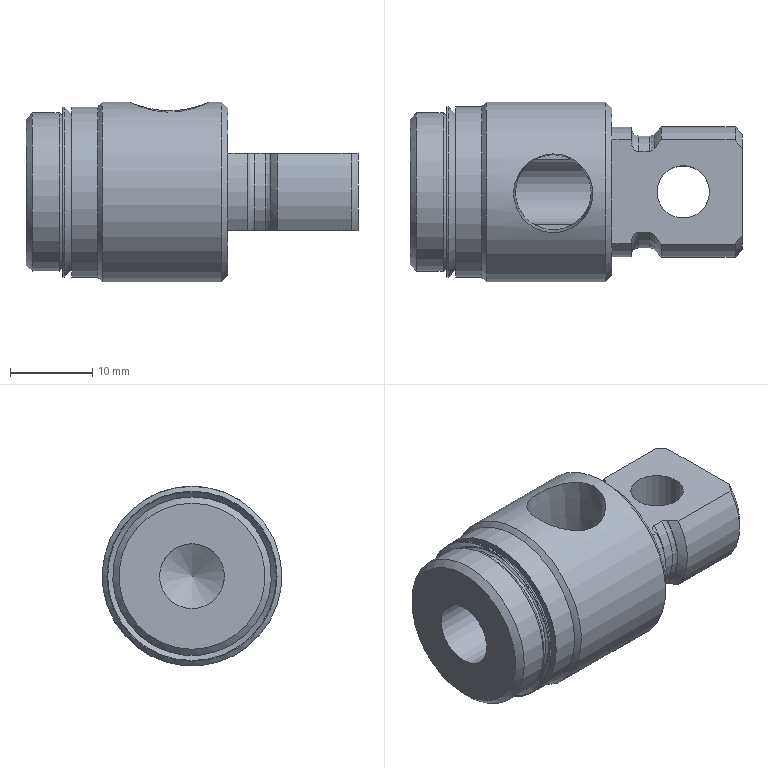Part | NX | features solid 2 | 1 solid | 46 faces | box 40.488 x 21.908 x 21.908 mm | volume 8739 mm3 | cylinder 15 | cone 15 | plane 11 | torus 5 | commonest cylinder face diameters 9.2 x2 13.678 x2 15.812 x2 15.875 x2 20.752 x2 6.401 x1
STEP:
#1=CARTESIAN_POINT('',(27.,6.111,-4.731));
#2=VERTEX_POINT('',#1);
#3=CARTESIAN_POINT('',(27.,6.334,-4.731));
#4=VERTEX_POINT('',#3);
#5=CARTESIAN_POINT('',(27.,7.906,-4.731));
#6=DIRECTION('',(0.,1.,0.));
#7=VECTOR('',#6,1000.);
#8=LINE('',#5,#7);
#9=EDGE_CURVE('',#2,#4,#8,.T.);
#10=ORIENTED_EDGE('',*,*,#9,.F.);
#11=CARTESIAN_POINT('',(27.889,4.939,-4.731));
#12=VERTEX_POINT('',#11);
#13=CARTESIAN_POINT('',(27.,6.111,-4.731));
#14=CARTESIAN_POINT('',(27.,5.839,-4.731));
#15=CARTESIAN_POINT('',(27.138,5.302,-4.731));
#16=CARTESIAN_POINT('',(27.62,4.939,-4.731));
#17=CARTESIAN_POINT('',(27.889,4.939,-4.731));
#18=B_SPLINE_CURVE_WITH_KNOTS('',3,(#13,#14,#15,#16,#17),.UNSPECIFIED.,.F.,.F.,(4,1,4),(0.004854,0.005662,0.006469),.UNSPECIFIED.);
#19=EDGE_CURVE('',#2,#12,#18,.T.);
#20=ORIENTED_EDGE('',*,*,#19,.T.);
#21=CARTESIAN_POINT('',(29.172,4.939,-4.731));
#22=VERTEX_POINT('',#21);
#23=CARTESIAN_POINT('',(40.488,4.939,-4.731));
#24=DIRECTION('',(-1.,0.,0.));
#25=VECTOR('',#24,1000.);
#26=LINE('',#23,#25);
#27=EDGE_CURVE('',#22,#12,#26,.T.);
#28=ORIENTED_EDGE('',*,*,#27,.F.);
#29=CARTESIAN_POINT('',(29.771,5.255,-4.731));
#30=VERTEX_POINT('',#29);
#31=CARTESIAN_POINT('',(29.172,4.939,-4.731));
#32=CARTESIAN_POINT('',(29.404,4.939,-4.731));
#33=CARTESIAN_POINT('',(29.624,5.076,-4.731));
#34=CARTESIAN_POINT('',(29.771,5.255,-4.731));
#35=B_SPLINE_CURVE_WITH_KNOTS('',3,(#31,#32,#33,#34),.UNSPECIFIED.,.F.,.F.,(4,4),(0.00608,0.006774),.UNSPECIFIED.);
#36=EDGE_CURVE('',#22,#30,#35,.T.);
#37=ORIENTED_EDGE('',*,*,#36,.T.);
#38=CARTESIAN_POINT('',(29.801,5.292,-4.731));
#39=VERTEX_POINT('',#38);
#40=CARTESIAN_POINT('',(29.801,5.292,-4.731));
#41=CARTESIAN_POINT('',(29.791,5.279,-4.731));
#42=CARTESIAN_POINT('',(29.781,5.267,-4.731));
#43=CARTESIAN_POINT('',(29.771,5.255,-4.731));
#44=B_SPLINE_CURVE_WITH_KNOTS('',3,(#40,#41,#42,#43),.UNSPECIFIED.,.F.,.F.,(4,4),(0.01225,0.0123),.UNSPECIFIED.);
#45=EDGE_CURVE('',#39,#30,#44,.T.);
#46=ORIENTED_EDGE('',*,*,#45,.F.);
#47=CARTESIAN_POINT('',(30.64,6.374,-4.731));
#48=VERTEX_POINT('',#47);
#49=CARTESIAN_POINT('',(30.64,6.374,-4.731));
#50=CARTESIAN_POINT('',(30.354,6.018,-4.731));
#51=CARTESIAN_POINT('',(30.073,5.658,-4.731));
#52=CARTESIAN_POINT('',(29.801,5.292,-4.731));
#53=B_SPLINE_CURVE_WITH_KNOTS('',3,(#49,#50,#51,#52),.UNSPECIFIED.,.F.,.F.,(4,4),(0.01415,0.01552),.UNSPECIFIED.);
#54=EDGE_CURVE('',#48,#39,#53,.T.);
#55=ORIENTED_EDGE('',*,*,#54,.F.);
#56=CARTESIAN_POINT('',(39.648,6.374,-4.731));
#57=VERTEX_POINT('',#56);
#58=CARTESIAN_POINT('',(40.488,6.374,-4.731));
#59=DIRECTION('',(-1.,0.,0.));
#60=VECTOR('',#59,1000.);
#61=LINE('',#58,#60);
#62=EDGE_CURVE('',#57,#48,#61,.T.);
#63=ORIENTED_EDGE('',*,*,#62,.F.);
#64=CARTESIAN_POINT('',(40.488,5.292,-4.731));
#65=VERTEX_POINT('',#64);
#66=CARTESIAN_POINT('',(40.488,5.292,-4.731));
#67=CARTESIAN_POINT('',(40.215,5.657,-4.731));
#68=CARTESIAN_POINT('',(39.934,6.017,-4.731));
#69=CARTESIAN_POINT('',(39.648,6.374,-4.731));
#70=B_SPLINE_CURVE_WITH_KNOTS('',3,(#66,#67,#68,#69),.UNSPECIFIED.,.F.,.F.,(4,4),(0.02732,0.02869),.UNSPECIFIED.);
#71=EDGE_CURVE('',#65,#57,#70,.T.);
#72=ORIENTED_EDGE('',*,*,#71,.F.);
#73=CARTESIAN_POINT('',(40.488,-5.292,-4.731));
#74=VERTEX_POINT('',#73);
#75=CARTESIAN_POINT('',(40.488,-21.907,-4.731));
#76=DIRECTION('',(0.,1.,0.));
#77=VECTOR('',#76,1000.);
#78=LINE('',#75,#77);
#79=EDGE_CURVE('',#74,#65,#78,.T.);
#80=ORIENTED_EDGE('',*,*,#79,.F.);
#81=CARTESIAN_POINT('',(39.648,-6.374,-4.731));
#82=VERTEX_POINT('',#81);
#83=CARTESIAN_POINT('',(39.648,-6.374,-4.731));
#84=CARTESIAN_POINT('',(39.934,-6.018,-4.731));
#85=CARTESIAN_POINT('',(40.215,-5.658,-4.731));
#86=CARTESIAN_POINT('',(40.488,-5.292,-4.731));
#87=B_SPLINE_CURVE_WITH_KNOTS('',3,(#83,#84,#85,#86),.UNSPECIFIED.,.F.,.F.,(4,4),(0.01415,0.01552),.UNSPECIFIED.);
#88=EDGE_CURVE('',#82,#74,#87,.T.);
#89=ORIENTED_EDGE('',*,*,#88,.F.);
#90=CARTESIAN_POINT('',(30.64,-6.374,-4.731));
#91=VERTEX_POINT('',#90);
#92=CARTESIAN_POINT('',(40.488,-6.374,-4.731));
#93=DIRECTION('',(-1.,0.,0.));
#94=VECTOR('',#93,1000.);
#95=LINE('',#92,#94);
#96=EDGE_CURVE('',#91,#82,#95,.F.);
#97=ORIENTED_EDGE('',*,*,#96,.F.);
#98=CARTESIAN_POINT('',(29.801,-5.292,-4.731));
#99=VERTEX_POINT('',#98);
#100=CARTESIAN_POINT('',(29.801,-5.292,-4.731));
#101=CARTESIAN_POINT('',(30.073,-5.657,-4.731));
#102=CARTESIAN_POINT('',(30.354,-6.017,-4.731));
#103=CARTESIAN_POINT('',(30.64,-6.374,-4.731));
#104=B_SPLINE_CURVE_WITH_KNOTS('',3,(#100,#101,#102,#103),.UNSPECIFIED.,.F.,.F.,(4,4),(0.02732,0.02869),.UNSPECIFIED.);
#105=EDGE_CURVE('',#99,#91,#104,.T.);
#106=ORIENTED_EDGE('',*,*,#105,.F.);
#107=CARTESIAN_POINT('',(29.771,-5.255,-4.731));
#108=VERTEX_POINT('',#107);
#109=CARTESIAN_POINT('',(29.771,-5.255,-4.731));
#110=CARTESIAN_POINT('',(29.781,-5.267,-4.731));
#111=CARTESIAN_POINT('',(29.791,-5.279,-4.731));
#112=CARTESIAN_POINT('',(29.801,-5.292,-4.731));
#113=B_SPLINE_CURVE_WITH_KNOTS('',3,(#109,#110,#111,#112),.UNSPECIFIED.,.F.,.F.,(4,4),(0.02417,0.02422),.UNSPECIFIED.);
#114=EDGE_CURVE('',#108,#99,#113,.T.);
#115=ORIENTED_EDGE('',*,*,#114,.F.);
#116=CARTESIAN_POINT('',(29.172,-4.939,-4.731));
#117=VERTEX_POINT('',#116);
#118=CARTESIAN_POINT('',(29.771,-5.255,-4.731));
#119=CARTESIAN_POINT('',(29.624,-5.075,-4.731));
#120=CARTESIAN_POINT('',(29.405,-4.939,-4.731));
#121=CARTESIAN_POINT('',(29.172,-4.939,-4.731));
#122=B_SPLINE_CURVE_WITH_KNOTS('',3,(#118,#119,#120,#121),.UNSPECIFIED.,.F.,.F.,(4,4),(0.00183,0.002524),.UNSPECIFIED.);
#123=EDGE_CURVE('',#108,#117,#122,.T.);
#124=ORIENTED_EDGE('',*,*,#123,.T.);
#125=CARTESIAN_POINT('',(27.889,-4.939,-4.731));
#126=VERTEX_POINT('',#125);
#127=CARTESIAN_POINT('',(40.488,-4.939,-4.731));
#128=DIRECTION('',(-1.,0.,0.));
#129=VECTOR('',#128,1000.);
#130=LINE('',#127,#129);
#131=EDGE_CURVE('',#126,#117,#130,.F.);
#132=ORIENTED_EDGE('',*,*,#131,.F.);
#133=CARTESIAN_POINT('',(27.,-6.111,-4.731));
#134=VERTEX_POINT('',#133);
#135=CARTESIAN_POINT('',(27.889,-4.939,-4.731));
#136=CARTESIAN_POINT('',(27.62,-4.939,-4.731));
#137=CARTESIAN_POINT('',(27.139,-5.299,-4.731));
#138=CARTESIAN_POINT('',(27.,-5.843,-4.731));
#139=CARTESIAN_POINT('',(27.,-6.111,-4.731));
#140=B_SPLINE_CURVE_WITH_KNOTS('',3,(#135,#136,#137,#138,#139),.UNSPECIFIED.,.F.,.F.,(4,1,4),(0.003324,0.004131,0.004938),.UNSPECIFIED.);
#141=EDGE_CURVE('',#126,#134,#140,.T.);
#142=ORIENTED_EDGE('',*,*,#141,.T.);
#143=CARTESIAN_POINT('',(27.,-6.334,-4.731));
#144=VERTEX_POINT('',#143);
#145=CARTESIAN_POINT('',(27.,7.906,-4.731));
#146=DIRECTION('',(0.,1.,0.));
#147=VECTOR('',#146,1000.);
#148=LINE('',#145,#147);
#149=EDGE_CURVE('',#144,#134,#148,.T.);
#150=ORIENTED_EDGE('',*,*,#149,.F.);
#151=CARTESIAN_POINT('',(24.613,-6.334,-4.731));
#152=VERTEX_POINT('',#151);
#153=CARTESIAN_POINT('',(40.488,-6.334,-4.731));
#154=DIRECTION('',(-1.,0.,0.));
#155=VECTOR('',#154,1000.);
#156=LINE('',#153,#155);
#157=EDGE_CURVE('',#152,#144,#156,.F.);
#158=ORIENTED_EDGE('',*,*,#157,.F.);
#159=CARTESIAN_POINT('',(24.613,6.334,-4.731));
#160=VERTEX_POINT('',#159);
#161=CARTESIAN_POINT('',(24.613,-21.907,-4.731));
#162=DIRECTION('',(0.,1.,0.));
#163=VECTOR('',#162,1000.);
#164=LINE('',#161,#163);
#165=EDGE_CURVE('',#152,#160,#164,.T.);
#166=ORIENTED_EDGE('',*,*,#165,.T.);
#167=CARTESIAN_POINT('',(40.488,6.334,-4.731));
#168=DIRECTION('',(-1.,0.,0.));
#169=VECTOR('',#168,1000.);
#170=LINE('',#167,#169);
#171=EDGE_CURVE('',#4,#160,#170,.T.);
#172=ORIENTED_EDGE('',*,*,#171,.F.);
#173=EDGE_LOOP('',(#10,#20,#28,#37,#46,#55,#63,#72,#80,#89,#97,#106,#115,#124,#132,#142,#150,#158,#166,#172));
#174=FACE_BOUND('',#173,.T.);
#175=CARTESIAN_POINT('',(30.124,0.,-4.731));
#176=VERTEX_POINT('',#175);
#177=CARTESIAN_POINT('',(33.325,0.,-4.731));
#178=DIRECTION('',(0.,0.,-1.));
#179=DIRECTION('',(-1.,0.,0.));
#180=AXIS2_PLACEMENT_3D('',#177,#178,#179);
#181=CIRCLE('',#180,3.2);
#182=EDGE_CURVE('',#176,#176,#181,.F.);
#183=ORIENTED_EDGE('',*,*,#182,.T.);
#184=EDGE_LOOP('',(#183));
#185=FACE_BOUND('',#184,.T.);
#186=CARTESIAN_POINT('',(24.613,-21.907,-4.731));
#187=DIRECTION('',(0.,0.,-1.));
#188=DIRECTION('',(-1.,0.,0.));
#189=AXIS2_PLACEMENT_3D('',#186,#187,#188);
#190=PLANE('',#189);
#191=ADVANCED_FACE('',(#174,#185),#190,.T.);
#192=CARTESIAN_POINT('',(27.,-6.111,4.731));
#193=VERTEX_POINT('',#192);
#194=CARTESIAN_POINT('',(27.,-6.334,4.731));
#195=VERTEX_POINT('',#194);
#196=CARTESIAN_POINT('',(27.,7.906,4.731));
#197=DIRECTION('',(0.,-1.,0.));
#198=VECTOR('',#197,1000.);
#199=LINE('',#196,#198);
#200=EDGE_CURVE('',#193,#195,#199,.T.);
#201=ORIENTED_EDGE('',*,*,#200,.F.);
#202=CARTESIAN_POINT('',(27.889,-4.939,4.731));
#203=VERTEX_POINT('',#202);
#204=CARTESIAN_POINT('',(27.,-6.111,4.731));
#205=CARTESIAN_POINT('',(27.,-5.842,4.731));
#206=CARTESIAN_POINT('',(27.139,-5.3,4.731));
#207=CARTESIAN_POINT('',(27.619,-4.939,4.731));
#208=CARTESIAN_POINT('',(27.889,-4.939,4.731));
#209=B_SPLINE_CURVE_WITH_KNOTS('',3,(#204,#205,#206,#207,#208),.UNSPECIFIED.,.F.,.F.,(4,1,4),(0.001401,0.002207,0.003014),.UNSPECIFIED.);
#210=EDGE_CURVE('',#193,#203,#209,.T.);
#211=ORIENTED_EDGE('',*,*,#210,.T.);
#212=CARTESIAN_POINT('',(29.172,-4.939,4.731));
#213=VERTEX_POINT('',#212);
#214=CARTESIAN_POINT('',(40.488,-4.939,4.731));
#215=DIRECTION('',(-1.,0.,0.));
#216=VECTOR('',#215,1000.);
#217=LINE('',#214,#216);
#218=EDGE_CURVE('',#213,#203,#217,.T.);
#219=ORIENTED_EDGE('',*,*,#218,.F.);
#220=CARTESIAN_POINT('',(29.771,-5.255,4.731));
#221=VERTEX_POINT('',#220);
#222=CARTESIAN_POINT('',(29.172,-4.939,4.731));
#223=CARTESIAN_POINT('',(29.405,-4.939,4.731));
#224=CARTESIAN_POINT('',(29.622,-5.073,4.731));
#225=CARTESIAN_POINT('',(29.771,-5.255,4.731));
#226=B_SPLINE_CURVE_WITH_KNOTS('',3,(#222,#223,#224,#225),.UNSPECIFIED.,.F.,.F.,(4,4),(0.003812,0.004508),.UNSPECIFIED.);
#227=EDGE_CURVE('',#213,#221,#226,.T.);
#228=ORIENTED_EDGE('',*,*,#227,.T.);
#229=CARTESIAN_POINT('',(29.801,-5.292,4.731));
#230=VERTEX_POINT('',#229);
#231=CARTESIAN_POINT('',(29.801,-5.292,4.731));
#232=CARTESIAN_POINT('',(29.791,-5.279,4.731));
#233=CARTESIAN_POINT('',(29.781,-5.267,4.731));
#234=CARTESIAN_POINT('',(29.771,-5.255,4.731));
#235=B_SPLINE_CURVE_WITH_KNOTS('',3,(#231,#232,#233,#234),.UNSPECIFIED.,.F.,.F.,(4,4),(0.01225,0.0123),.UNSPECIFIED.);
#236=EDGE_CURVE('',#230,#221,#235,.T.);
#237=ORIENTED_EDGE('',*,*,#236,.F.);
#238=CARTESIAN_POINT('',(30.64,-6.374,4.731));
#239=VERTEX_POINT('',#238);
#240=CARTESIAN_POINT('',(30.64,-6.374,4.731));
#241=CARTESIAN_POINT('',(30.354,-6.018,4.731));
#242=CARTESIAN_POINT('',(30.073,-5.658,4.731));
#243=CARTESIAN_POINT('',(29.801,-5.292,4.731));
#244=B_SPLINE_CURVE_WITH_KNOTS('',3,(#240,#241,#242,#243),.UNSPECIFIED.,.F.,.F.,(4,4),(0.01415,0.01552),.UNSPECIFIED.);
#245=EDGE_CURVE('',#239,#230,#244,.T.);
#246=ORIENTED_EDGE('',*,*,#245,.F.);
#247=CARTESIAN_POINT('',(39.648,-6.374,4.731));
#248=VERTEX_POINT('',#247);
#249=CARTESIAN_POINT('',(40.488,-6.374,4.731));
#250=DIRECTION('',(-1.,0.,0.));
#251=VECTOR('',#250,1000.);
#252=LINE('',#249,#251);
#253=EDGE_CURVE('',#248,#239,#252,.T.);
#254=ORIENTED_EDGE('',*,*,#253,.F.);
#255=CARTESIAN_POINT('',(40.488,-5.292,4.731));
#256=VERTEX_POINT('',#255);
#257=CARTESIAN_POINT('',(40.488,-5.292,4.731));
#258=CARTESIAN_POINT('',(40.215,-5.657,4.731));
#259=CARTESIAN_POINT('',(39.934,-6.017,4.731));
#260=CARTESIAN_POINT('',(39.648,-6.374,4.731));
#261=B_SPLINE_CURVE_WITH_KNOTS('',3,(#257,#258,#259,#260),.UNSPECIFIED.,.F.,.F.,(4,4),(0.02732,0.02869),.UNSPECIFIED.);
#262=EDGE_CURVE('',#256,#248,#261,.T.);
#263=ORIENTED_EDGE('',*,*,#262,.F.);
#264=CARTESIAN_POINT('',(40.488,5.292,4.731));
#265=VERTEX_POINT('',#264);
#266=CARTESIAN_POINT('',(40.488,21.907,4.731));
#267=DIRECTION('',(0.,-1.,0.));
#268=VECTOR('',#267,1000.);
#269=LINE('',#266,#268);
#270=EDGE_CURVE('',#265,#256,#269,.T.);
#271=ORIENTED_EDGE('',*,*,#270,.F.);
#272=CARTESIAN_POINT('',(39.648,6.374,4.731));
#273=VERTEX_POINT('',#272);
#274=CARTESIAN_POINT('',(39.648,6.374,4.731));
#275=CARTESIAN_POINT('',(39.934,6.018,4.731));
#276=CARTESIAN_POINT('',(40.215,5.658,4.731));
#277=CARTESIAN_POINT('',(40.488,5.292,4.731));
#278=B_SPLINE_CURVE_WITH_KNOTS('',3,(#274,#275,#276,#277),.UNSPECIFIED.,.F.,.F.,(4,4),(0.01415,0.01552),.UNSPECIFIED.);
#279=EDGE_CURVE('',#273,#265,#278,.T.);
#280=ORIENTED_EDGE('',*,*,#279,.F.);
#281=CARTESIAN_POINT('',(30.64,6.374,4.731));
#282=VERTEX_POINT('',#281);
#283=CARTESIAN_POINT('',(40.488,6.374,4.731));
#284=DIRECTION('',(-1.,0.,0.));
#285=VECTOR('',#284,1000.);
#286=LINE('',#283,#285);
#287=EDGE_CURVE('',#282,#273,#286,.F.);
#288=ORIENTED_EDGE('',*,*,#287,.F.);
#289=CARTESIAN_POINT('',(29.801,5.292,4.731));
#290=VERTEX_POINT('',#289);
#291=CARTESIAN_POINT('',(29.801,5.292,4.731));
#292=CARTESIAN_POINT('',(30.073,5.657,4.731));
#293=CARTESIAN_POINT('',(30.354,6.017,4.731));
#294=CARTESIAN_POINT('',(30.64,6.374,4.731));
#295=B_SPLINE_CURVE_WITH_KNOTS('',3,(#291,#292,#293,#294),.UNSPECIFIED.,.F.,.F.,(4,4),(0.02732,0.02869),.UNSPECIFIED.);
#296=EDGE_CURVE('',#290,#282,#295,.T.);
#297=ORIENTED_EDGE('',*,*,#296,.F.);
#298=CARTESIAN_POINT('',(29.771,5.255,4.731));
#299=VERTEX_POINT('',#298);
#300=CARTESIAN_POINT('',(29.771,5.255,4.731));
#301=CARTESIAN_POINT('',(29.781,5.267,4.731));
#302=CARTESIAN_POINT('',(29.791,5.279,4.731));
#303=CARTESIAN_POINT('',(29.801,5.292,4.731));
#304=B_SPLINE_CURVE_WITH_KNOTS('',3,(#300,#301,#302,#303),.UNSPECIFIED.,.F.,.F.,(4,4),(0.02417,0.02422),.UNSPECIFIED.);
#305=EDGE_CURVE('',#299,#290,#304,.T.);
#306=ORIENTED_EDGE('',*,*,#305,.F.);
#307=CARTESIAN_POINT('',(29.172,4.939,4.731));
#308=VERTEX_POINT('',#307);
#309=CARTESIAN_POINT('',(29.771,5.255,4.731));
#310=CARTESIAN_POINT('',(29.623,5.075,4.731));
#311=CARTESIAN_POINT('',(29.406,4.939,4.731));
#312=CARTESIAN_POINT('',(29.172,4.939,4.731));
#313=B_SPLINE_CURVE_WITH_KNOTS('',3,(#309,#310,#311,#312),.UNSPECIFIED.,.F.,.F.,(4,4),(0.005905,0.0066),.UNSPECIFIED.);
#314=EDGE_CURVE('',#299,#308,#313,.T.);
#315=ORIENTED_EDGE('',*,*,#314,.T.);
#316=CARTESIAN_POINT('',(27.889,4.939,4.731));
#317=VERTEX_POINT('',#316);
#318=CARTESIAN_POINT('',(40.488,4.939,4.731));
#319=DIRECTION('',(-1.,0.,0.));
#320=VECTOR('',#319,1000.);
#321=LINE('',#318,#320);
#322=EDGE_CURVE('',#317,#308,#321,.F.);
#323=ORIENTED_EDGE('',*,*,#322,.F.);
#324=CARTESIAN_POINT('',(27.,6.111,4.731));
#325=VERTEX_POINT('',#324);
#326=CARTESIAN_POINT('',(27.889,4.939,4.731));
#327=CARTESIAN_POINT('',(27.62,4.939,4.731));
#328=CARTESIAN_POINT('',(27.139,5.299,4.731));
#329=CARTESIAN_POINT('',(27.,5.842,4.731));
#330=CARTESIAN_POINT('',(27.,6.111,4.731));
#331=B_SPLINE_CURVE_WITH_KNOTS('',3,(#326,#327,#328,#329,#330),.UNSPECIFIED.,.F.,.F.,(4,1,4),(0.006205,0.007011,0.007818),.UNSPECIFIED.);
#332=EDGE_CURVE('',#317,#325,#331,.T.);
#333=ORIENTED_EDGE('',*,*,#332,.T.);
#334=CARTESIAN_POINT('',(27.,6.334,4.731));
#335=VERTEX_POINT('',#334);
#336=CARTESIAN_POINT('',(27.,7.906,4.731));
#337=DIRECTION('',(0.,-1.,0.));
#338=VECTOR('',#337,1000.);
#339=LINE('',#336,#338);
#340=EDGE_CURVE('',#335,#325,#339,.T.);
#341=ORIENTED_EDGE('',*,*,#340,.F.);
#342=CARTESIAN_POINT('',(24.613,6.334,4.731));
#343=VERTEX_POINT('',#342);
#344=CARTESIAN_POINT('',(40.488,6.334,4.731));
#345=DIRECTION('',(-1.,0.,0.));
#346=VECTOR('',#345,1000.);
#347=LINE('',#344,#346);
#348=EDGE_CURVE('',#343,#335,#347,.F.);
#349=ORIENTED_EDGE('',*,*,#348,.F.);
#350=CARTESIAN_POINT('',(24.613,-6.334,4.731));
#351=VERTEX_POINT('',#350);
#352=CARTESIAN_POINT('',(24.613,21.907,4.731));
#353=DIRECTION('',(0.,-1.,0.));
#354=VECTOR('',#353,1000.);
#355=LINE('',#352,#354);
#356=EDGE_CURVE('',#343,#351,#355,.T.);
#357=ORIENTED_EDGE('',*,*,#356,.T.);
#358=CARTESIAN_POINT('',(40.488,-6.334,4.731));
#359=DIRECTION('',(-1.,0.,0.));
#360=VECTOR('',#359,1000.);
#361=LINE('',#358,#360);
#362=EDGE_CURVE('',#195,#351,#361,.T.);
#363=ORIENTED_EDGE('',*,*,#362,.F.);
#364=EDGE_LOOP('',(#201,#211,#219,#228,#237,#246,#254,#263,#271,#280,#288,#297,#306,#315,#323,#333,#341,#349,#357,#363));
#365=FACE_BOUND('',#364,.T.);
#366=CARTESIAN_POINT('',(36.525,0.,4.731));
#367=VERTEX_POINT('',#366);
#368=CARTESIAN_POINT('',(33.325,0.,4.731));
#369=DIRECTION('',(0.,0.,1.));
#370=DIRECTION('',(1.,0.,0.));
#371=AXIS2_PLACEMENT_3D('',#368,#369,#370);
#372=CIRCLE('',#371,3.2);
#373=EDGE_CURVE('',#367,#367,#372,.F.);
#374=ORIENTED_EDGE('',*,*,#373,.T.);
#375=EDGE_LOOP('',(#374));
#376=FACE_BOUND('',#375,.T.);
#377=CARTESIAN_POINT('',(24.613,21.907,4.731));
#378=DIRECTION('',(0.,0.,1.));
#379=DIRECTION('',(1.,0.,0.));
#380=AXIS2_PLACEMENT_3D('',#377,#378,#379);
#381=PLANE('',#380);
#382=ADVANCED_FACE('',(#365,#376),#381,.T.);
#383=CARTESIAN_POINT('',(4.801,0.,8.909));
#384=VERTEX_POINT('',#383);
#385=CARTESIAN_POINT('',(4.801,0.,0.));
#386=DIRECTION('',(-1.,0.,0.));
#387=DIRECTION('',(0.,0.,1.));
#388=AXIS2_PLACEMENT_3D('',#385,#386,#387);
#389=CIRCLE('',#388,8.909);
#390=EDGE_CURVE('',#384,#384,#389,.T.);
#391=ORIENTED_EDGE('',*,*,#390,.F.);
#392=EDGE_LOOP('',(#391));
#393=FACE_BOUND('',#392,.T.);
#394=CARTESIAN_POINT('',(5.182,0.,8.909));
#395=VERTEX_POINT('',#394);
#396=CARTESIAN_POINT('',(5.182,0.,0.));
#397=DIRECTION('',(-1.,0.,0.));
#398=DIRECTION('',(0.,0.,1.));
#399=AXIS2_PLACEMENT_3D('',#396,#397,#398);
#400=CIRCLE('',#399,8.909);
#401=EDGE_CURVE('',#395,#395,#400,.T.);
#402=ORIENTED_EDGE('',*,*,#401,.T.);
#403=EDGE_LOOP('',(#402));
#404=FACE_BOUND('',#403,.T.);
#405=CARTESIAN_POINT('',(24.613,0.,0.));
#406=DIRECTION('',(-1.,0.,0.));
#407=DIRECTION('',(0.,0.,1.));
#408=AXIS2_PLACEMENT_3D('',#405,#406,#407);
#409=CYLINDRICAL_SURFACE('',#408,8.909);
#410=ADVANCED_FACE('',(#393,#404),#409,.T.);
#411=CARTESIAN_POINT('',(5.563,0.,10.376));
#412=VERTEX_POINT('',#411);
#413=CARTESIAN_POINT('',(5.563,0.,0.));
#414=DIRECTION('',(-1.,0.,0.));
#415=DIRECTION('',(0.,0.,1.));
#416=AXIS2_PLACEMENT_3D('',#413,#414,#415);
#417=CIRCLE('',#416,10.376);
#418=EDGE_CURVE('',#412,#412,#417,.T.);
#419=ORIENTED_EDGE('',*,*,#418,.T.);
#420=EDGE_LOOP('',(#419));
#421=FACE_BOUND('',#420,.T.);
#422=CARTESIAN_POINT('',(5.563,0.,9.512));
#423=VERTEX_POINT('',#422);
#424=CARTESIAN_POINT('',(5.563,0.,0.));
#425=DIRECTION('',(-1.,0.,0.));
#426=DIRECTION('',(0.,0.,1.));
#427=AXIS2_PLACEMENT_3D('',#424,#425,#426);
#428=CIRCLE('',#427,9.512);
#429=EDGE_CURVE('',#423,#423,#428,.T.);
#430=ORIENTED_EDGE('',*,*,#429,.F.);
#431=EDGE_LOOP('',(#430));
#432=FACE_BOUND('',#431,.T.);
#433=CARTESIAN_POINT('',(5.563,8.909,0.));
#434=DIRECTION('',(-1.,0.,0.));
#435=DIRECTION('',(0.,0.,1.));
#436=AXIS2_PLACEMENT_3D('',#433,#434,#435);
#437=PLANE('',#436);
#438=ADVANCED_FACE('',(#421,#432),#437,.T.);
#439=ORIENTED_EDGE('',*,*,#227,.F.);
#440=CARTESIAN_POINT('',(29.172,0.,0.));
#441=DIRECTION('',(-1.,0.,0.));
#442=DIRECTION('',(0.,0.,1.));
#443=AXIS2_PLACEMENT_3D('',#440,#441,#442);
#444=CIRCLE('',#443,6.839);
#445=EDGE_CURVE('',#117,#213,#444,.T.);
#446=ORIENTED_EDGE('',*,*,#445,.F.);
#447=ORIENTED_EDGE('',*,*,#123,.F.);
#448=CARTESIAN_POINT('',(29.771,0.,0.));
#449=DIRECTION('',(-1.,0.,0.));
#450=DIRECTION('',(0.,0.,1.));
#451=AXIS2_PLACEMENT_3D('',#448,#449,#450);
#452=CIRCLE('',#451,7.071);
#453=EDGE_CURVE('',#108,#221,#452,.T.);
#454=ORIENTED_EDGE('',*,*,#453,.T.);
#455=EDGE_LOOP('',(#439,#446,#447,#454));
#456=FACE_BOUND('',#455,.T.);
#457=CARTESIAN_POINT('',(29.172,0.,0.));
#458=DIRECTION('',(-1.,0.,0.));
#459=DIRECTION('',(0.,0.,1.));
#460=AXIS2_PLACEMENT_3D('',#457,#458,#459);
#461=TOROIDAL_SURFACE('',#460,7.728,0.889);
#462=ADVANCED_FACE('',(#456),#461,.F.);
#463=ORIENTED_EDGE('',*,*,#314,.F.);
#464=CARTESIAN_POINT('',(29.771,0.,0.));
#465=DIRECTION('',(-1.,0.,0.));
#466=DIRECTION('',(0.,0.,1.));
#467=AXIS2_PLACEMENT_3D('',#464,#465,#466);
#468=CIRCLE('',#467,7.071);
#469=EDGE_CURVE('',#299,#30,#468,.T.);
#470=ORIENTED_EDGE('',*,*,#469,.T.);
#471=ORIENTED_EDGE('',*,*,#36,.F.);
#472=CARTESIAN_POINT('',(29.172,0.,0.));
#473=DIRECTION('',(-1.,0.,0.));
#474=DIRECTION('',(0.,0.,1.));
#475=AXIS2_PLACEMENT_3D('',#472,#473,#474);
#476=CIRCLE('',#475,6.839);
#477=EDGE_CURVE('',#308,#22,#476,.T.);
#478=ORIENTED_EDGE('',*,*,#477,.F.);
#479=EDGE_LOOP('',(#463,#470,#471,#478));
#480=FACE_BOUND('',#479,.T.);
#481=CARTESIAN_POINT('',(29.172,0.,0.));
#482=DIRECTION('',(-1.,0.,0.));
#483=DIRECTION('',(0.,0.,1.));
#484=AXIS2_PLACEMENT_3D('',#481,#482,#483);
#485=TOROIDAL_SURFACE('',#484,7.728,0.889);
#486=ADVANCED_FACE('',(#480),#485,.F.);
#487=CARTESIAN_POINT('',(27.889,0.,0.));
#488=DIRECTION('',(-1.,0.,0.));
#489=DIRECTION('',(0.,0.,1.));
#490=AXIS2_PLACEMENT_3D('',#487,#488,#489);
#491=CIRCLE('',#490,6.839);
#492=EDGE_CURVE('',#317,#12,#491,.T.);
#493=ORIENTED_EDGE('',*,*,#492,.F.);
#494=ORIENTED_EDGE('',*,*,#322,.T.);
#495=ORIENTED_EDGE('',*,*,#477,.T.);
#496=ORIENTED_EDGE('',*,*,#27,.T.);
#497=EDGE_LOOP('',(#493,#494,#495,#496));
#498=FACE_BOUND('',#497,.T.);
#499=CARTESIAN_POINT('',(40.488,0.,0.));
#500=DIRECTION('',(-1.,0.,0.));
#501=DIRECTION('',(0.,0.,1.));
#502=AXIS2_PLACEMENT_3D('',#499,#500,#501);
#503=CYLINDRICAL_SURFACE('',#502,6.839);
#504=ADVANCED_FACE('',(#498),#503,.T.);
#505=ORIENTED_EDGE('',*,*,#445,.T.);
#506=ORIENTED_EDGE('',*,*,#218,.T.);
#507=CARTESIAN_POINT('',(27.889,0.,0.));
#508=DIRECTION('',(-1.,0.,0.));
#509=DIRECTION('',(0.,0.,1.));
#510=AXIS2_PLACEMENT_3D('',#507,#508,#509);
#511=CIRCLE('',#510,6.839);
#512=EDGE_CURVE('',#126,#203,#511,.T.);
#513=ORIENTED_EDGE('',*,*,#512,.F.);
#514=ORIENTED_EDGE('',*,*,#131,.T.);
#515=EDGE_LOOP('',(#505,#506,#513,#514));
#516=FACE_BOUND('',#515,.T.);
#517=CARTESIAN_POINT('',(40.488,0.,0.));
#518=DIRECTION('',(-1.,0.,0.));
#519=DIRECTION('',(0.,0.,1.));
#520=AXIS2_PLACEMENT_3D('',#517,#518,#519);
#521=CYLINDRICAL_SURFACE('',#520,6.839);
#522=ADVANCED_FACE('',(#516),#521,.T.);
#523=ORIENTED_EDGE('',*,*,#210,.F.);
#524=CARTESIAN_POINT('',(27.,0.,0.));
#525=DIRECTION('',(-1.,0.,0.));
#526=DIRECTION('',(0.,0.,1.));
#527=AXIS2_PLACEMENT_3D('',#524,#525,#526);
#528=CIRCLE('',#527,7.728);
#529=EDGE_CURVE('',#134,#193,#528,.T.);
#530=ORIENTED_EDGE('',*,*,#529,.F.);
#531=ORIENTED_EDGE('',*,*,#141,.F.);
#532=ORIENTED_EDGE('',*,*,#512,.T.);
#533=EDGE_LOOP('',(#523,#530,#531,#532));
#534=FACE_BOUND('',#533,.T.);
#535=CARTESIAN_POINT('',(27.889,0.,0.));
#536=DIRECTION('',(-1.,0.,0.));
#537=DIRECTION('',(0.,0.,1.));
#538=AXIS2_PLACEMENT_3D('',#535,#536,#537);
#539=TOROIDAL_SURFACE('',#538,7.728,0.889);
#540=ADVANCED_FACE('',(#534),#539,.F.);
#541=ORIENTED_EDGE('',*,*,#332,.F.);
#542=ORIENTED_EDGE('',*,*,#492,.T.);
#543=ORIENTED_EDGE('',*,*,#19,.F.);
#544=CARTESIAN_POINT('',(27.,0.,0.));
#545=DIRECTION('',(-1.,0.,0.));
#546=DIRECTION('',(0.,0.,1.));
#547=AXIS2_PLACEMENT_3D('',#544,#545,#546);
#548=CIRCLE('',#547,7.728);
#549=EDGE_CURVE('',#325,#2,#548,.T.);
#550=ORIENTED_EDGE('',*,*,#549,.F.);
#551=EDGE_LOOP('',(#541,#542,#543,#550));
#552=FACE_BOUND('',#551,.T.);
#553=CARTESIAN_POINT('',(27.889,0.,0.));
#554=DIRECTION('',(-1.,0.,0.));
#555=DIRECTION('',(0.,0.,1.));
#556=AXIS2_PLACEMENT_3D('',#553,#554,#555);
#557=TOROIDAL_SURFACE('',#556,7.728,0.889);
#558=ADVANCED_FACE('',(#552),#557,.F.);
#559=CARTESIAN_POINT('',(27.,0.,0.));
#560=DIRECTION('',(-1.,0.,0.));
#561=DIRECTION('',(0.,0.,1.));
#562=AXIS2_PLACEMENT_3D('',#559,#560,#561);
#563=CIRCLE('',#562,7.906);
#564=EDGE_CURVE('',#335,#4,#563,.T.);
#565=ORIENTED_EDGE('',*,*,#564,.F.);
#566=ORIENTED_EDGE('',*,*,#340,.T.);
#567=ORIENTED_EDGE('',*,*,#549,.T.);
#568=ORIENTED_EDGE('',*,*,#9,.T.);
#569=EDGE_LOOP('',(#565,#566,#567,#568));
#570=FACE_BOUND('',#569,.T.);
#571=CARTESIAN_POINT('',(27.,7.906,0.));
#572=DIRECTION('',(1.,0.,0.));
#573=DIRECTION('',(0.,0.,-1.));
#574=AXIS2_PLACEMENT_3D('',#571,#572,#573);
#575=PLANE('',#574);
#576=ADVANCED_FACE('',(#570),#575,.T.);
#577=ORIENTED_EDGE('',*,*,#529,.T.);
#578=ORIENTED_EDGE('',*,*,#200,.T.);
#579=CARTESIAN_POINT('',(27.,0.,0.));
#580=DIRECTION('',(-1.,0.,0.));
#581=DIRECTION('',(0.,0.,1.));
#582=AXIS2_PLACEMENT_3D('',#579,#580,#581);
#583=CIRCLE('',#582,7.906);
#584=EDGE_CURVE('',#144,#195,#583,.T.);
#585=ORIENTED_EDGE('',*,*,#584,.F.);
#586=ORIENTED_EDGE('',*,*,#149,.T.);
#587=EDGE_LOOP('',(#577,#578,#585,#586));
#588=FACE_BOUND('',#587,.T.);
#589=CARTESIAN_POINT('',(27.,7.906,0.));
#590=DIRECTION('',(1.,0.,0.));
#591=DIRECTION('',(0.,0.,-1.));
#592=AXIS2_PLACEMENT_3D('',#589,#590,#591);
#593=PLANE('',#592);
#594=ADVANCED_FACE('',(#588),#593,.T.);
#595=CARTESIAN_POINT('',(24.613,0.,0.));
#596=DIRECTION('',(1.,0.,0.));
#597=DIRECTION('',(0.,0.,-1.));
#598=AXIS2_PLACEMENT_3D('',#595,#596,#597);
#599=CIRCLE('',#598,7.906);
#600=EDGE_CURVE('',#160,#343,#599,.T.);
#601=ORIENTED_EDGE('',*,*,#600,.T.);
#602=ORIENTED_EDGE('',*,*,#348,.T.);
#603=ORIENTED_EDGE('',*,*,#564,.T.);
#604=ORIENTED_EDGE('',*,*,#171,.T.);
#605=EDGE_LOOP('',(#601,#602,#603,#604));
#606=FACE_BOUND('',#605,.T.);
#607=CARTESIAN_POINT('',(40.488,0.,0.));
#608=DIRECTION('',(-1.,0.,0.));
#609=DIRECTION('',(0.,0.,1.));
#610=AXIS2_PLACEMENT_3D('',#607,#608,#609);
#611=CYLINDRICAL_SURFACE('',#610,7.906);
#612=ADVANCED_FACE('',(#606),#611,.T.);
#613=ORIENTED_EDGE('',*,*,#584,.T.);
#614=ORIENTED_EDGE('',*,*,#362,.T.);
#615=CARTESIAN_POINT('',(24.613,0.,0.));
#616=DIRECTION('',(1.,0.,0.));
#617=DIRECTION('',(0.,0.,-1.));
#618=AXIS2_PLACEMENT_3D('',#615,#616,#617);
#619=CIRCLE('',#618,7.906);
#620=EDGE_CURVE('',#351,#152,#619,.T.);
#621=ORIENTED_EDGE('',*,*,#620,.T.);
#622=ORIENTED_EDGE('',*,*,#157,.T.);
#623=EDGE_LOOP('',(#613,#614,#621,#622));
#624=FACE_BOUND('',#623,.T.);
#625=CARTESIAN_POINT('',(40.488,0.,0.));
#626=DIRECTION('',(-1.,0.,0.));
#627=DIRECTION('',(0.,0.,1.));
#628=AXIS2_PLACEMENT_3D('',#625,#626,#627);
#629=CYLINDRICAL_SURFACE('',#628,7.906);
#630=ADVANCED_FACE('',(#624),#629,.T.);
#631=CARTESIAN_POINT('',(40.488,0.,0.));
#632=DIRECTION('',(-1.,0.,0.));
#633=DIRECTION('',(0.,0.,1.));
#634=AXIS2_PLACEMENT_3D('',#631,#632,#633);
#635=CIRCLE('',#634,7.098);
#636=EDGE_CURVE('',#265,#65,#635,.T.);
#637=ORIENTED_EDGE('',*,*,#636,.F.);
#638=ORIENTED_EDGE('',*,*,#270,.T.);
#639=CARTESIAN_POINT('',(40.488,0.,0.));
#640=DIRECTION('',(-1.,0.,0.));
#641=DIRECTION('',(0.,0.,1.));
#642=AXIS2_PLACEMENT_3D('',#639,#640,#641);
#643=CIRCLE('',#642,7.098);
#644=EDGE_CURVE('',#74,#256,#643,.T.);
#645=ORIENTED_EDGE('',*,*,#644,.F.);
#646=ORIENTED_EDGE('',*,*,#79,.T.);
#647=EDGE_LOOP('',(#637,#638,#645,#646));
#648=FACE_BOUND('',#647,.T.);
#649=CARTESIAN_POINT('',(40.488,7.098,0.));
#650=DIRECTION('',(1.,0.,0.));
#651=DIRECTION('',(0.,0.,-1.));
#652=AXIS2_PLACEMENT_3D('',#649,#650,#651);
#653=PLANE('',#652);
#654=ADVANCED_FACE('',(#648),#653,.T.);
#655=CARTESIAN_POINT('',(39.648,0.,0.));
#656=DIRECTION('',(-1.,0.,0.));
#657=DIRECTION('',(0.,0.,1.));
#658=AXIS2_PLACEMENT_3D('',#655,#656,#657);
#659=CIRCLE('',#658,7.938);
#660=EDGE_CURVE('',#273,#57,#659,.T.);
#661=ORIENTED_EDGE('',*,*,#660,.F.);
#662=ORIENTED_EDGE('',*,*,#279,.T.);
#663=ORIENTED_EDGE('',*,*,#636,.T.);
#664=ORIENTED_EDGE('',*,*,#71,.T.);
#665=EDGE_LOOP('',(#661,#662,#663,#664));
#666=FACE_BOUND('',#665,.T.);
#667=CARTESIAN_POINT('',(39.648,0.,0.));
#668=DIRECTION('',(-1.,0.,0.));
#669=DIRECTION('',(0.,0.,1.));
#670=AXIS2_PLACEMENT_3D('',#667,#668,#669);
#671=CONICAL_SURFACE('',#670,7.938,0.7854);
#672=ADVANCED_FACE('',(#666),#671,.T.);
#673=ORIENTED_EDGE('',*,*,#644,.T.);
#674=ORIENTED_EDGE('',*,*,#262,.T.);
#675=CARTESIAN_POINT('',(39.648,0.,0.));
#676=DIRECTION('',(-1.,0.,0.));
#677=DIRECTION('',(0.,0.,1.));
#678=AXIS2_PLACEMENT_3D('',#675,#676,#677);
#679=CIRCLE('',#678,7.938);
#680=EDGE_CURVE('',#82,#248,#679,.T.);
#681=ORIENTED_EDGE('',*,*,#680,.F.);
#682=ORIENTED_EDGE('',*,*,#88,.T.);
#683=EDGE_LOOP('',(#673,#674,#681,#682));
#684=FACE_BOUND('',#683,.T.);
#685=CARTESIAN_POINT('',(39.648,0.,0.));
#686=DIRECTION('',(-1.,0.,0.));
#687=DIRECTION('',(0.,0.,1.));
#688=AXIS2_PLACEMENT_3D('',#685,#686,#687);
#689=CONICAL_SURFACE('',#688,7.938,0.7854);
#690=ADVANCED_FACE('',(#684),#689,.T.);
#691=CARTESIAN_POINT('',(30.64,0.,0.));
#692=DIRECTION('',(-1.,0.,0.));
#693=DIRECTION('',(0.,0.,1.));
#694=AXIS2_PLACEMENT_3D('',#691,#692,#693);
#695=CIRCLE('',#694,7.938);
#696=EDGE_CURVE('',#282,#48,#695,.T.);
#697=ORIENTED_EDGE('',*,*,#696,.F.);
#698=ORIENTED_EDGE('',*,*,#287,.T.);
#699=ORIENTED_EDGE('',*,*,#660,.T.);
#700=ORIENTED_EDGE('',*,*,#62,.T.);
#701=EDGE_LOOP('',(#697,#698,#699,#700));
#702=FACE_BOUND('',#701,.T.);
#703=CARTESIAN_POINT('',(40.488,0.,0.));
#704=DIRECTION('',(-1.,0.,0.));
#705=DIRECTION('',(0.,0.,1.));
#706=AXIS2_PLACEMENT_3D('',#703,#704,#705);
#707=CYLINDRICAL_SURFACE('',#706,7.938);
#708=ADVANCED_FACE('',(#702),#707,.T.);
#709=ORIENTED_EDGE('',*,*,#680,.T.);
#710=ORIENTED_EDGE('',*,*,#253,.T.);
#711=CARTESIAN_POINT('',(30.64,0.,0.));
#712=DIRECTION('',(-1.,0.,0.));
#713=DIRECTION('',(0.,0.,1.));
#714=AXIS2_PLACEMENT_3D('',#711,#712,#713);
#715=CIRCLE('',#714,7.938);
#716=EDGE_CURVE('',#91,#239,#715,.T.);
#717=ORIENTED_EDGE('',*,*,#716,.F.);
#718=ORIENTED_EDGE('',*,*,#96,.T.);
#719=EDGE_LOOP('',(#709,#710,#717,#718));
#720=FACE_BOUND('',#719,.T.);
#721=CARTESIAN_POINT('',(40.488,0.,0.));
#722=DIRECTION('',(-1.,0.,0.));
#723=DIRECTION('',(0.,0.,1.));
#724=AXIS2_PLACEMENT_3D('',#721,#722,#723);
#725=CYLINDRICAL_SURFACE('',#724,7.938);
#726=ADVANCED_FACE('',(#720),#725,.T.);
#727=ORIENTED_EDGE('',*,*,#716,.T.);
#728=ORIENTED_EDGE('',*,*,#245,.T.);
#729=CARTESIAN_POINT('',(29.801,0.,0.));
#730=DIRECTION('',(-1.,0.,0.));
#731=DIRECTION('',(0.,0.,1.));
#732=AXIS2_PLACEMENT_3D('',#729,#730,#731);
#733=CIRCLE('',#732,7.098);
#734=EDGE_CURVE('',#99,#230,#733,.T.);
#735=ORIENTED_EDGE('',*,*,#734,.F.);
#736=ORIENTED_EDGE('',*,*,#105,.T.);
#737=EDGE_LOOP('',(#727,#728,#735,#736));
#738=FACE_BOUND('',#737,.T.);
#739=CARTESIAN_POINT('',(29.801,0.,0.));
#740=DIRECTION('',(1.,0.,0.));
#741=DIRECTION('',(0.,0.,-1.));
#742=AXIS2_PLACEMENT_3D('',#739,#740,#741);
#743=CONICAL_SURFACE('',#742,7.098,0.7854);
#744=ADVANCED_FACE('',(#738),#743,.T.);
#745=CARTESIAN_POINT('',(29.801,0.,0.));
#746=DIRECTION('',(-1.,0.,0.));
#747=DIRECTION('',(0.,0.,1.));
#748=AXIS2_PLACEMENT_3D('',#745,#746,#747);
#749=CIRCLE('',#748,7.098);
#750=EDGE_CURVE('',#290,#39,#749,.T.);
#751=ORIENTED_EDGE('',*,*,#750,.F.);
#752=ORIENTED_EDGE('',*,*,#296,.T.);
#753=ORIENTED_EDGE('',*,*,#696,.T.);
#754=ORIENTED_EDGE('',*,*,#54,.T.);
#755=EDGE_LOOP('',(#751,#752,#753,#754));
#756=FACE_BOUND('',#755,.T.);
#757=CARTESIAN_POINT('',(29.801,0.,0.));
#758=DIRECTION('',(1.,0.,0.));
#759=DIRECTION('',(0.,0.,-1.));
#760=AXIS2_PLACEMENT_3D('',#757,#758,#759);
#761=CONICAL_SURFACE('',#760,7.098,0.7854);
#762=ADVANCED_FACE('',(#756),#761,.T.);
#763=ORIENTED_EDGE('',*,*,#734,.T.);
#764=ORIENTED_EDGE('',*,*,#236,.T.);
#765=ORIENTED_EDGE('',*,*,#453,.F.);
#766=ORIENTED_EDGE('',*,*,#114,.T.);
#767=EDGE_LOOP('',(#763,#764,#765,#766));
#768=FACE_BOUND('',#767,.T.);
#769=CARTESIAN_POINT('',(29.771,0.,0.));
#770=DIRECTION('',(1.,0.,0.));
#771=DIRECTION('',(0.,0.,-1.));
#772=AXIS2_PLACEMENT_3D('',#769,#770,#771);
#773=CONICAL_SURFACE('',#772,7.071,0.7389);
#774=ADVANCED_FACE('',(#768),#773,.T.);
#775=ORIENTED_EDGE('',*,*,#469,.F.);
#776=ORIENTED_EDGE('',*,*,#305,.T.);
#777=ORIENTED_EDGE('',*,*,#750,.T.);
#778=ORIENTED_EDGE('',*,*,#45,.T.);
#779=EDGE_LOOP('',(#775,#776,#777,#778));
#780=FACE_BOUND('',#779,.T.);
#781=CARTESIAN_POINT('',(29.771,0.,0.));
#782=DIRECTION('',(1.,0.,0.));
#783=DIRECTION('',(0.,0.,-1.));
#784=AXIS2_PLACEMENT_3D('',#781,#782,#783);
#785=CONICAL_SURFACE('',#784,7.071,0.7389);
#786=ADVANCED_FACE('',(#780),#785,.T.);
#787=CARTESIAN_POINT('',(0.762,0.,9.671));
#788=VERTEX_POINT('',#787);
#789=CARTESIAN_POINT('',(0.762,0.,0.));
#790=DIRECTION('',(-1.,0.,0.));
#791=DIRECTION('',(0.,0.,1.));
#792=AXIS2_PLACEMENT_3D('',#789,#790,#791);
#793=CIRCLE('',#792,9.671);
#794=EDGE_CURVE('',#788,#788,#793,.T.);
#795=ORIENTED_EDGE('',*,*,#794,.T.);
#796=EDGE_LOOP('',(#795));
#797=FACE_BOUND('',#796,.T.);
#798=CARTESIAN_POINT('',(0.,0.,8.909));
#799=VERTEX_POINT('',#798);
#800=CARTESIAN_POINT('',(0.,0.,0.));
#801=DIRECTION('',(-1.,0.,0.));
#802=DIRECTION('',(0.,0.,1.));
#803=AXIS2_PLACEMENT_3D('',#800,#801,#802);
#804=CIRCLE('',#803,8.909);
#805=EDGE_CURVE('',#799,#799,#804,.T.);
#806=ORIENTED_EDGE('',*,*,#805,.F.);
#807=EDGE_LOOP('',(#806));
#808=FACE_BOUND('',#807,.T.);
#809=CARTESIAN_POINT('',(0.,0.,0.));
#810=DIRECTION('',(1.,0.,0.));
#811=DIRECTION('',(0.,0.,-1.));
#812=AXIS2_PLACEMENT_3D('',#809,#810,#811);
#813=CONICAL_SURFACE('',#812,8.909,0.7854);
#814=ADVANCED_FACE('',(#797,#808),#813,.T.);
#815=CARTESIAN_POINT('',(4.039,0.,9.671));
#816=VERTEX_POINT('',#815);
#817=CARTESIAN_POINT('',(4.039,0.,0.));
#818=DIRECTION('',(-1.,0.,0.));
#819=DIRECTION('',(0.,0.,1.));
#820=AXIS2_PLACEMENT_3D('',#817,#818,#819);
#821=CIRCLE('',#820,9.671);
#822=EDGE_CURVE('',#816,#816,#821,.T.);
#823=ORIENTED_EDGE('',*,*,#822,.T.);
#824=EDGE_LOOP('',(#823));
#825=FACE_BOUND('',#824,.T.);
#826=ORIENTED_EDGE('',*,*,#794,.F.);
#827=EDGE_LOOP('',(#826));
#828=FACE_BOUND('',#827,.T.);
#829=CARTESIAN_POINT('',(24.613,0.,0.));
#830=DIRECTION('',(-1.,0.,0.));
#831=DIRECTION('',(0.,0.,1.));
#832=AXIS2_PLACEMENT_3D('',#829,#830,#831);
#833=CYLINDRICAL_SURFACE('',#832,9.671);
#834=ADVANCED_FACE('',(#825,#828),#833,.T.);
#835=ORIENTED_EDGE('',*,*,#390,.T.);
#836=EDGE_LOOP('',(#835));
#837=FACE_BOUND('',#836,.T.);
#838=ORIENTED_EDGE('',*,*,#822,.F.);
#839=EDGE_LOOP('',(#838));
#840=FACE_BOUND('',#839,.T.);
#841=CARTESIAN_POINT('',(4.039,0.,0.));
#842=DIRECTION('',(-1.,0.,0.));
#843=DIRECTION('',(0.,0.,1.));
#844=AXIS2_PLACEMENT_3D('',#841,#842,#843);
#845=CONICAL_SURFACE('',#844,9.671,0.7854);
#846=ADVANCED_FACE('',(#837,#840),#845,.T.);
#847=CARTESIAN_POINT('',(8.736,0.,10.376));
#848=VERTEX_POINT('',#847);
#849=CARTESIAN_POINT('',(8.736,0.,0.));
#850=DIRECTION('',(-1.,0.,0.));
#851=DIRECTION('',(0.,0.,1.));
#852=AXIS2_PLACEMENT_3D('',#849,#850,#851);
#853=CIRCLE('',#852,10.376);
#854=EDGE_CURVE('',#848,#848,#853,.T.);
#855=ORIENTED_EDGE('',*,*,#854,.T.);
#856=EDGE_LOOP('',(#855));
#857=FACE_BOUND('',#856,.T.);
#858=ORIENTED_EDGE('',*,*,#418,.F.);
#859=EDGE_LOOP('',(#858));
#860=FACE_BOUND('',#859,.T.);
#861=CARTESIAN_POINT('',(24.613,0.,0.));
#862=DIRECTION('',(-1.,0.,0.));
#863=DIRECTION('',(0.,0.,1.));
#864=AXIS2_PLACEMENT_3D('',#861,#862,#863);
#865=CYLINDRICAL_SURFACE('',#864,10.376);
#866=ADVANCED_FACE('',(#857,#860),#865,.T.);
#867=CARTESIAN_POINT('',(9.314,0.,10.954));
#868=VERTEX_POINT('',#867);
#869=CARTESIAN_POINT('',(9.314,0.,0.));
#870=DIRECTION('',(-1.,0.,0.));
#871=DIRECTION('',(0.,0.,1.));
#872=AXIS2_PLACEMENT_3D('',#869,#870,#871);
#873=CIRCLE('',#872,10.954);
#874=EDGE_CURVE('',#868,#868,#873,.T.);
#875=ORIENTED_EDGE('',*,*,#874,.T.);
#876=EDGE_LOOP('',(#875));
#877=FACE_BOUND('',#876,.T.);
#878=ORIENTED_EDGE('',*,*,#854,.F.);
#879=EDGE_LOOP('',(#878));
#880=FACE_BOUND('',#879,.T.);
#881=CARTESIAN_POINT('',(8.736,0.,0.));
#882=DIRECTION('',(1.,0.,0.));
#883=DIRECTION('',(0.,0.,-1.));
#884=AXIS2_PLACEMENT_3D('',#881,#882,#883);
#885=CONICAL_SURFACE('',#884,10.376,0.7854);
#886=ADVANCED_FACE('',(#877,#880),#885,.T.);
#887=CARTESIAN_POINT('',(14.133,-3.656,10.326));
#888=VERTEX_POINT('',#887);
#889=CARTESIAN_POINT('',(12.106,-0.2961,11.216));
#890=CARTESIAN_POINT('',(13.776,-4.04,10.319));
#891=CARTESIAN_POINT('',(17.586,-5.481,9.461));
#892=CARTESIAN_POINT('',(21.329,-3.886,10.39));
#893=CARTESIAN_POINT('',(22.843,-0.08836,11.218));
#894=CARTESIAN_POINT('',(21.18,3.667,10.457));
#895=CARTESIAN_POINT('',(17.374,5.15,9.646));
#896=CARTESIAN_POINT('',(13.621,3.52,10.519));
#897=CARTESIAN_POINT('',(12.106,-0.2961,11.216));
#898=CARTESIAN_POINT('',(13.776,-4.04,10.319));
#899=CARTESIAN_POINT('',(17.586,-5.481,9.461));
#900=B_SPLINE_CURVE_WITH_KNOTS('',3,(#889,#890,#891,#892,#893,#894,#895,#896,#897,#898,#899),.UNSPECIFIED.,.T.,.F.,(1,1,1,1,1,1,1,1,1,1,1,1,1,1,1),(-0.01145,-0.007634,-0.003817,0.,0.003817,0.007634,0.01145,0.01527,0.01908,0.0229,0.02672,0.03054,0.03435,0.03817,0.04199),.UNSPECIFIED.);
#901=EDGE_CURVE('',#888,#888,#900,.T.);
#902=ORIENTED_EDGE('',*,*,#901,.F.);
#903=EDGE_LOOP('',(#902));
#904=FACE_BOUND('',#903,.T.);
#905=CARTESIAN_POINT('',(23.851,0.,10.954));
#906=VERTEX_POINT('',#905);
#907=CARTESIAN_POINT('',(23.851,0.,0.));
#908=DIRECTION('',(-1.,0.,0.));
#909=DIRECTION('',(0.,0.,1.));
#910=AXIS2_PLACEMENT_3D('',#907,#908,#909);
#911=CIRCLE('',#910,10.954);
#912=EDGE_CURVE('',#906,#906,#911,.T.);
#913=ORIENTED_EDGE('',*,*,#912,.T.);
#914=EDGE_LOOP('',(#913));
#915=FACE_BOUND('',#914,.T.);
#916=ORIENTED_EDGE('',*,*,#874,.F.);
#917=EDGE_LOOP('',(#916));
#918=FACE_BOUND('',#917,.T.);
#919=CARTESIAN_POINT('',(24.613,0.,0.));
#920=DIRECTION('',(-1.,0.,0.));
#921=DIRECTION('',(0.,0.,1.));
#922=AXIS2_PLACEMENT_3D('',#919,#920,#921);
#923=CYLINDRICAL_SURFACE('',#922,10.954);
#924=ADVANCED_FACE('',(#904,#915,#918),#923,.T.);
#925=CARTESIAN_POINT('',(24.613,0.,10.192));
#926=VERTEX_POINT('',#925);
#927=CARTESIAN_POINT('',(24.613,0.,0.));
#928=DIRECTION('',(-1.,0.,0.));
#929=DIRECTION('',(0.,0.,1.));
#930=AXIS2_PLACEMENT_3D('',#927,#928,#929);
#931=CIRCLE('',#930,10.192);
#932=EDGE_CURVE('',#926,#926,#931,.T.);
#933=ORIENTED_EDGE('',*,*,#932,.T.);
#934=EDGE_LOOP('',(#933));
#935=FACE_BOUND('',#934,.T.);
#936=ORIENTED_EDGE('',*,*,#912,.F.);
#937=EDGE_LOOP('',(#936));
#938=FACE_BOUND('',#937,.T.);
#939=CARTESIAN_POINT('',(23.851,0.,0.));
#940=DIRECTION('',(-1.,0.,0.));
#941=DIRECTION('',(0.,0.,1.));
#942=AXIS2_PLACEMENT_3D('',#939,#940,#941);
#943=CONICAL_SURFACE('',#942,10.954,0.7854);
#944=ADVANCED_FACE('',(#935,#938),#943,.T.);
#945=ORIENTED_EDGE('',*,*,#356,.F.);
#946=ORIENTED_EDGE('',*,*,#600,.F.);
#947=ORIENTED_EDGE('',*,*,#165,.F.);
#948=ORIENTED_EDGE('',*,*,#620,.F.);
#949=EDGE_LOOP('',(#945,#946,#947,#948));
#950=FACE_BOUND('',#949,.T.);
#951=ORIENTED_EDGE('',*,*,#932,.F.);
#952=EDGE_LOOP('',(#951));
#953=FACE_BOUND('',#952,.T.);
#954=CARTESIAN_POINT('',(24.613,10.192,0.));
#955=DIRECTION('',(1.,0.,0.));
#956=DIRECTION('',(0.,0.,-1.));
#957=AXIS2_PLACEMENT_3D('',#954,#955,#956);
#958=PLANE('',#957);
#959=ADVANCED_FACE('',(#950,#953),#958,.T.);
#960=CARTESIAN_POINT('',(0.,0.,-3.962));
#961=VERTEX_POINT('',#960);
#962=CARTESIAN_POINT('',(0.,0.,0.));
#963=DIRECTION('',(1.,0.,0.));
#964=DIRECTION('',(0.,0.,-1.));
#965=AXIS2_PLACEMENT_3D('',#962,#963,#964);
#966=CIRCLE('',#965,3.962);
#967=EDGE_CURVE('',#961,#961,#966,.T.);
#968=ORIENTED_EDGE('',*,*,#967,.T.);
#969=EDGE_LOOP('',(#968));
#970=FACE_BOUND('',#969,.T.);
#971=ORIENTED_EDGE('',*,*,#805,.T.);
#972=EDGE_LOOP('',(#971));
#973=FACE_BOUND('',#972,.T.);
#974=CARTESIAN_POINT('',(0.,0.,0.));
#975=DIRECTION('',(-1.,0.,0.));
#976=DIRECTION('',(0.,0.,1.));
#977=AXIS2_PLACEMENT_3D('',#974,#975,#976);
#978=PLANE('',#977);
#979=ADVANCED_FACE('',(#970,#973),#978,.T.);
#980=CARTESIAN_POINT('',(23.581,0.,-3.962));
#981=VERTEX_POINT('',#980);
#982=CARTESIAN_POINT('',(23.581,0.,0.));
#983=DIRECTION('',(1.,0.,0.));
#984=DIRECTION('',(0.,0.,-1.));
#985=AXIS2_PLACEMENT_3D('',#982,#983,#984);
#986=CIRCLE('',#985,3.962);
#987=EDGE_CURVE('',#981,#981,#986,.T.);
#988=ORIENTED_EDGE('',*,*,#987,.F.);
#989=EDGE_LOOP('',(#988));
#990=FACE_BOUND('',#989,.T.);
#991=CARTESIAN_POINT('',(25.869,0.,0.));
#992=VERTEX_POINT('',#991);
#993=VERTEX_LOOP('',#992);
#994=FACE_BOUND('',#993,.T.);
#995=CARTESIAN_POINT('',(23.581,0.,0.));
#996=DIRECTION('',(-1.,0.,0.));
#997=DIRECTION('',(0.,0.,1.));
#998=AXIS2_PLACEMENT_3D('',#995,#996,#997);
#999=CONICAL_SURFACE('',#998,3.962,1.047);
#1000=ADVANCED_FACE('',(#990,#994),#999,.F.);
#1001=CARTESIAN_POINT('',(19.812,-3.962,-0.06915));
#1002=VERTEX_POINT('',#1001);
#1003=CARTESIAN_POINT('',(21.505,-2.276,3.244));
#1004=VERTEX_POINT('',#1003);
#1005=CARTESIAN_POINT('',(19.812,-3.962,-0.06915));
#1006=CARTESIAN_POINT('',(19.812,-3.974,0.6513));
#1007=CARTESIAN_POINT('',(20.48,-3.614,1.944));
#1008=CARTESIAN_POINT('',(21.208,-2.809,2.87));
#1009=CARTESIAN_POINT('',(21.505,-2.276,3.244));
#1010=B_SPLINE_CURVE_WITH_KNOTS('',3,(#1005,#1006,#1007,#1008,#1009),.UNSPECIFIED.,.F.,.F.,(4,1,4),(0.,0.002124,0.004248),.UNSPECIFIED.);
#1011=EDGE_CURVE('',#1002,#1004,#1010,.T.);
#1012=ORIENTED_EDGE('',*,*,#1011,.T.);
#1013=CARTESIAN_POINT('',(21.505,2.161,3.321));
#1014=VERTEX_POINT('',#1013);
#1015=CARTESIAN_POINT('',(21.505,-2.276,3.244));
#1016=CARTESIAN_POINT('',(21.857,-1.67,3.669));
#1017=CARTESIAN_POINT('',(22.336,-0.08007,4.227));
#1018=CARTESIAN_POINT('',(21.857,1.541,3.725));
#1019=CARTESIAN_POINT('',(21.505,2.161,3.321));
#1020=B_SPLINE_CURVE_WITH_KNOTS('',3,(#1015,#1016,#1017,#1018,#1019),.UNSPECIFIED.,.F.,.F.,(4,1,4),(0.00007889,0.002517,0.004956),.UNSPECIFIED.);
#1021=EDGE_CURVE('',#1004,#1014,#1020,.T.);
#1022=ORIENTED_EDGE('',*,*,#1021,.T.);
#1023=CARTESIAN_POINT('',(19.812,3.962,0.06915));
#1024=VERTEX_POINT('',#1023);
#1025=CARTESIAN_POINT('',(21.505,2.161,3.321));
#1026=CARTESIAN_POINT('',(21.207,2.708,2.965));
#1027=CARTESIAN_POINT('',(20.481,3.543,2.069));
#1028=CARTESIAN_POINT('',(19.812,3.949,0.7922));
#1029=CARTESIAN_POINT('',(19.812,3.962,0.06915));
#1030=B_SPLINE_CURVE_WITH_KNOTS('',3,(#1025,#1026,#1027,#1028,#1029),.UNSPECIFIED.,.F.,.F.,(4,1,4),(0.,0.002116,0.004232),.UNSPECIFIED.);
#1031=EDGE_CURVE('',#1014,#1024,#1030,.T.);
#1032=ORIENTED_EDGE('',*,*,#1031,.T.);
#1033=CARTESIAN_POINT('',(15.139,3.962,0.06915));
#1034=VERTEX_POINT('',#1033);
#1035=CARTESIAN_POINT('',(0.,3.962,0.06915));
#1036=DIRECTION('',(1.,0.,0.));
#1037=VECTOR('',#1036,1000.);
#1038=LINE('',#1035,#1037);
#1039=EDGE_CURVE('',#1024,#1034,#1038,.F.);
#1040=ORIENTED_EDGE('',*,*,#1039,.T.);
#1041=CARTESIAN_POINT('',(13.446,2.161,3.321));
#1042=VERTEX_POINT('',#1041);
#1043=CARTESIAN_POINT('',(15.139,3.962,0.06915));
#1044=CARTESIAN_POINT('',(15.139,3.949,0.7896));
#1045=CARTESIAN_POINT('',(14.47,3.544,2.069));
#1046=CARTESIAN_POINT('',(13.743,2.707,2.966));
#1047=CARTESIAN_POINT('',(13.446,2.161,3.321));
#1048=B_SPLINE_CURVE_WITH_KNOTS('',3,(#1043,#1044,#1045,#1046,#1047),.UNSPECIFIED.,.F.,.F.,(4,1,4),(0.,0.002124,0.004248),.UNSPECIFIED.);
#1049=EDGE_CURVE('',#1034,#1042,#1048,.T.);
#1050=ORIENTED_EDGE('',*,*,#1049,.T.);
#1051=CARTESIAN_POINT('',(13.446,-2.276,3.244));
#1052=VERTEX_POINT('',#1051);
#1053=CARTESIAN_POINT('',(13.446,2.161,3.321));
#1054=CARTESIAN_POINT('',(13.095,1.544,3.723));
#1055=CARTESIAN_POINT('',(12.614,-0.06776,4.227));
#1056=CARTESIAN_POINT('',(13.092,-1.668,3.67));
#1057=CARTESIAN_POINT('',(13.446,-2.276,3.244));
#1058=B_SPLINE_CURVE_WITH_KNOTS('',3,(#1053,#1054,#1055,#1056,#1057),.UNSPECIFIED.,.F.,.F.,(4,1,4),(0.0002324,0.002671,0.005109),.UNSPECIFIED.);
#1059=EDGE_CURVE('',#1042,#1052,#1058,.T.);
#1060=ORIENTED_EDGE('',*,*,#1059,.T.);
#1061=CARTESIAN_POINT('',(15.139,-3.962,-0.06915));
#1062=VERTEX_POINT('',#1061);
#1063=CARTESIAN_POINT('',(13.446,-2.276,3.244));
#1064=CARTESIAN_POINT('',(13.743,-2.81,2.869));
#1065=CARTESIAN_POINT('',(14.469,-3.613,1.944));
#1066=CARTESIAN_POINT('',(15.139,-3.974,0.6539));
#1067=CARTESIAN_POINT('',(15.139,-3.962,-0.06915));
#1068=B_SPLINE_CURVE_WITH_KNOTS('',3,(#1063,#1064,#1065,#1066,#1067),.UNSPECIFIED.,.F.,.F.,(4,1,4),(0.,0.002116,0.004232),.UNSPECIFIED.);
#1069=EDGE_CURVE('',#1052,#1062,#1068,.T.);
#1070=ORIENTED_EDGE('',*,*,#1069,.T.);
#1071=CARTESIAN_POINT('',(0.,-3.962,-0.06915));
#1072=DIRECTION('',(1.,0.,0.));
#1073=VECTOR('',#1072,1000.);
#1074=LINE('',#1071,#1073);
#1075=EDGE_CURVE('',#1062,#1002,#1074,.T.);
#1076=ORIENTED_EDGE('',*,*,#1075,.T.);
#1077=EDGE_LOOP('',(#1012,#1022,#1032,#1040,#1050,#1060,#1070,#1076));
#1078=FACE_BOUND('',#1077,.T.);
#1079=ORIENTED_EDGE('',*,*,#987,.T.);
#1080=EDGE_LOOP('',(#1079));
#1081=FACE_BOUND('',#1080,.T.);
#1082=ORIENTED_EDGE('',*,*,#967,.F.);
#1083=EDGE_LOOP('',(#1082));
#1084=FACE_BOUND('',#1083,.T.);
#1085=CARTESIAN_POINT('',(0.,0.,0.));
#1086=DIRECTION('',(1.,0.,0.));
#1087=DIRECTION('',(0.,0.,-1.));
#1088=AXIS2_PLACEMENT_3D('',#1085,#1086,#1087);
#1089=CYLINDRICAL_SURFACE('',#1088,3.962);
#1090=ADVANCED_FACE('',(#1078,#1081,#1084),#1089,.F.);
#1091=CARTESIAN_POINT('',(17.475,0.,0.));
#1092=DIRECTION('',(0.,0.01745,-0.9998));
#1093=DIRECTION('',(0.,0.9998,0.01745));
#1094=AXIS2_PLACEMENT_3D('',#1091,#1092,#1093);
#1095=CIRCLE('',#1094,4.6);
#1096=EDGE_CURVE('',#1034,#1024,#1095,.T.);
#1097=ORIENTED_EDGE('',*,*,#1096,.F.);
#1098=ORIENTED_EDGE('',*,*,#1039,.F.);
#1099=EDGE_LOOP('',(#1097,#1098));
#1100=FACE_BOUND('',#1099,.T.);
#1101=CARTESIAN_POINT('',(17.475,0.,0.));
#1102=DIRECTION('',(0.,0.01745,-0.9998));
#1103=DIRECTION('',(0.,0.9998,0.01745));
#1104=AXIS2_PLACEMENT_3D('',#1101,#1102,#1103);
#1105=PLANE('',#1104);
#1106=ADVANCED_FACE('',(#1100),#1105,.F.);
#1107=CARTESIAN_POINT('',(17.475,0.,0.));
#1108=DIRECTION('',(0.,0.01745,-0.9998));
#1109=DIRECTION('',(0.,0.9998,0.01745));
#1110=AXIS2_PLACEMENT_3D('',#1107,#1108,#1109);
#1111=CIRCLE('',#1110,4.6);
#1112=EDGE_CURVE('',#1002,#1062,#1111,.T.);
#1113=ORIENTED_EDGE('',*,*,#1112,.F.);
#1114=ORIENTED_EDGE('',*,*,#1075,.F.);
#1115=EDGE_LOOP('',(#1113,#1114));
#1116=FACE_BOUND('',#1115,.T.);
#1117=CARTESIAN_POINT('',(17.475,0.,0.));
#1118=DIRECTION('',(0.,0.01745,-0.9998));
#1119=DIRECTION('',(0.,0.9998,0.01745));
#1120=AXIS2_PLACEMENT_3D('',#1117,#1118,#1119);
#1121=PLANE('',#1120);
#1122=ADVANCED_FACE('',(#1116),#1121,.F.);
#1123=CARTESIAN_POINT('',(17.475,-0.05729,3.282));
#1124=DIRECTION('',(0.,0.01745,-0.9998));
#1125=DIRECTION('',(0.,0.9998,0.01745));
#1126=AXIS2_PLACEMENT_3D('',#1123,#1124,#1125);
#1127=CIRCLE('',#1126,4.6);
#1128=EDGE_CURVE('',#1042,#1014,#1127,.T.);
#1129=ORIENTED_EDGE('',*,*,#1128,.F.);
#1130=ORIENTED_EDGE('',*,*,#1049,.F.);
#1131=ORIENTED_EDGE('',*,*,#1096,.T.);
#1132=ORIENTED_EDGE('',*,*,#1031,.F.);
#1133=EDGE_LOOP('',(#1129,#1130,#1131,#1132));
#1134=FACE_BOUND('',#1133,.T.);
#1135=CARTESIAN_POINT('',(17.475,0.,0.));
#1136=DIRECTION('',(0.,0.01745,-0.9998));
#1137=DIRECTION('',(0.,0.9998,0.01745));
#1138=AXIS2_PLACEMENT_3D('',#1135,#1136,#1137);
#1139=CYLINDRICAL_SURFACE('',#1138,4.6);
#1140=ADVANCED_FACE('',(#1134),#1139,.F.);
#1141=CARTESIAN_POINT('',(17.475,-0.05729,3.282));
#1142=DIRECTION('',(0.,0.01745,-0.9998));
#1143=DIRECTION('',(0.,0.9998,0.01745));
#1144=AXIS2_PLACEMENT_3D('',#1141,#1142,#1143);
#1145=CIRCLE('',#1144,4.6);
#1146=EDGE_CURVE('',#1004,#1052,#1145,.T.);
#1147=ORIENTED_EDGE('',*,*,#1146,.F.);
#1148=ORIENTED_EDGE('',*,*,#1011,.F.);
#1149=ORIENTED_EDGE('',*,*,#1112,.T.);
#1150=ORIENTED_EDGE('',*,*,#1069,.F.);
#1151=EDGE_LOOP('',(#1147,#1148,#1149,#1150));
#1152=FACE_BOUND('',#1151,.T.);
#1153=CARTESIAN_POINT('',(17.475,0.,0.));
#1154=DIRECTION('',(0.,0.01745,-0.9998));
#1155=DIRECTION('',(0.,0.9998,0.01745));
#1156=AXIS2_PLACEMENT_3D('',#1153,#1154,#1155);
#1157=CYLINDRICAL_SURFACE('',#1156,4.6);
#1158=ADVANCED_FACE('',(#1152),#1157,.F.);
#1159=ORIENTED_EDGE('',*,*,#901,.T.);
#1160=EDGE_LOOP('',(#1159));
#1161=FACE_BOUND('',#1160,.T.);
#1162=ORIENTED_EDGE('',*,*,#1146,.T.);
#1163=ORIENTED_EDGE('',*,*,#1059,.F.);
#1164=ORIENTED_EDGE('',*,*,#1128,.T.);
#1165=ORIENTED_EDGE('',*,*,#1021,.F.);
#1166=EDGE_LOOP('',(#1162,#1163,#1164,#1165));
#1167=FACE_BOUND('',#1166,.T.);
#1168=CARTESIAN_POINT('',(17.475,-0.1912,10.952));
#1169=DIRECTION('',(0.,-0.01745,0.9998));
#1170=DIRECTION('',(0.,-0.9998,-0.01745));
#1171=AXIS2_PLACEMENT_3D('',#1168,#1169,#1170);
#1172=CONICAL_SURFACE('',#1171,4.839,0.03121);
#1173=ADVANCED_FACE('',(#1161,#1167),#1172,.F.);
#1174=CARTESIAN_POINT('',(4.699,0.,10.376));
#1175=VERTEX_POINT('',#1174);
#1176=CARTESIAN_POINT('',(4.699,0.,0.));
#1177=DIRECTION('',(-1.,0.,0.));
#1178=DIRECTION('',(0.,0.,1.));
#1179=AXIS2_PLACEMENT_3D('',#1176,#1177,#1178);
#1180=CIRCLE('',#1179,10.376);
#1181=EDGE_CURVE('',#1175,#1175,#1180,.T.);
#1182=ORIENTED_EDGE('',*,*,#1181,.F.);
#1183=EDGE_LOOP('',(#1182));
#1184=FACE_BOUND('',#1183,.T.);
#1185=ORIENTED_EDGE('',*,*,#429,.T.);
#1186=EDGE_LOOP('',(#1185));
#1187=FACE_BOUND('',#1186,.T.);
#1188=CARTESIAN_POINT('',(5.563,0.,0.));
#1189=DIRECTION('',(-1.,0.,0.));
#1190=DIRECTION('',(0.,0.,1.));
#1191=AXIS2_PLACEMENT_3D('',#1188,#1189,#1190);
#1192=CONICAL_SURFACE('',#1191,9.512,0.7854);
#1193=ADVANCED_FACE('',(#1184,#1187),#1192,.T.);
#1194=CARTESIAN_POINT('',(4.496,0.,10.376));
#1195=VERTEX_POINT('',#1194);
#1196=CARTESIAN_POINT('',(4.496,0.,0.));
#1197=DIRECTION('',(-1.,0.,0.));
#1198=DIRECTION('',(0.,0.,1.));
#1199=AXIS2_PLACEMENT_3D('',#1196,#1197,#1198);
#1200=CIRCLE('',#1199,10.376);
#1201=EDGE_CURVE('',#1195,#1195,#1200,.T.);
#1202=ORIENTED_EDGE('',*,*,#1201,.F.);
#1203=EDGE_LOOP('',(#1202));
#1204=FACE_BOUND('',#1203,.T.);
#1205=ORIENTED_EDGE('',*,*,#1181,.T.);
#1206=EDGE_LOOP('',(#1205));
#1207=FACE_BOUND('',#1206,.T.);
#1208=CARTESIAN_POINT('',(5.563,0.,0.));
#1209=DIRECTION('',(-1.,0.,0.));
#1210=DIRECTION('',(0.,0.,1.));
#1211=AXIS2_PLACEMENT_3D('',#1208,#1209,#1210);
#1212=CYLINDRICAL_SURFACE('',#1211,10.376);
#1213=ADVANCED_FACE('',(#1204,#1207),#1212,.T.);
#1214=CARTESIAN_POINT('',(4.496,0.,10.292));
#1215=VERTEX_POINT('',#1214);
#1216=CARTESIAN_POINT('',(4.496,0.,0.));
#1217=DIRECTION('',(-1.,0.,0.));
#1218=DIRECTION('',(0.,0.,1.));
#1219=AXIS2_PLACEMENT_3D('',#1216,#1217,#1218);
#1220=CIRCLE('',#1219,10.292);
#1221=EDGE_CURVE('',#1215,#1215,#1220,.T.);
#1222=ORIENTED_EDGE('',*,*,#1221,.F.);
#1223=EDGE_LOOP('',(#1222));
#1224=FACE_BOUND('',#1223,.T.);
#1225=ORIENTED_EDGE('',*,*,#1201,.T.);
#1226=EDGE_LOOP('',(#1225));
#1227=FACE_BOUND('',#1226,.T.);
#1228=CARTESIAN_POINT('',(4.496,10.376,0.));
#1229=DIRECTION('',(1.,0.,0.));
#1230=DIRECTION('',(0.,0.,-1.));
#1231=AXIS2_PLACEMENT_3D('',#1228,#1229,#1230);
#1232=PLANE('',#1231);
#1233=ADVANCED_FACE('',(#1224,#1227),#1232,.F.);
#1234=CARTESIAN_POINT('',(5.44,0.,9.347));
#1235=VERTEX_POINT('',#1234);
#1236=CARTESIAN_POINT('',(5.44,0.,0.));
#1237=DIRECTION('',(-1.,0.,0.));
#1238=DIRECTION('',(0.,0.,1.));
#1239=AXIS2_PLACEMENT_3D('',#1236,#1237,#1238);
#1240=CIRCLE('',#1239,9.347);
#1241=EDGE_CURVE('',#1235,#1235,#1240,.T.);
#1242=ORIENTED_EDGE('',*,*,#1241,.F.);
#1243=EDGE_LOOP('',(#1242));
#1244=FACE_BOUND('',#1243,.T.);
#1245=ORIENTED_EDGE('',*,*,#1221,.T.);
#1246=EDGE_LOOP('',(#1245));
#1247=FACE_BOUND('',#1246,.T.);
#1248=CARTESIAN_POINT('',(4.496,0.,0.));
#1249=DIRECTION('',(-1.,0.,0.));
#1250=DIRECTION('',(0.,0.,1.));
#1251=AXIS2_PLACEMENT_3D('',#1248,#1249,#1250);
#1252=CONICAL_SURFACE('',#1251,10.292,0.7854);
#1253=ADVANCED_FACE('',(#1244,#1247),#1252,.F.);
#1254=ORIENTED_EDGE('',*,*,#1241,.T.);
#1255=EDGE_LOOP('',(#1254));
#1256=FACE_BOUND('',#1255,.T.);
#1257=CARTESIAN_POINT('',(5.44,0.,9.168));
#1258=VERTEX_POINT('',#1257);
#1259=CARTESIAN_POINT('',(5.44,0.,0.));
#1260=DIRECTION('',(-1.,0.,0.));
#1261=DIRECTION('',(0.,0.,1.));
#1262=AXIS2_PLACEMENT_3D('',#1259,#1260,#1261);
#1263=CIRCLE('',#1262,9.168);
#1264=EDGE_CURVE('',#1258,#1258,#1263,.T.);
#1265=ORIENTED_EDGE('',*,*,#1264,.F.);
#1266=EDGE_LOOP('',(#1265));
#1267=FACE_BOUND('',#1266,.T.);
#1268=CARTESIAN_POINT('',(5.35,0.,0.));
#1269=DIRECTION('',(-1.,0.,0.));
#1270=DIRECTION('',(0.,0.,1.));
#1271=AXIS2_PLACEMENT_3D('',#1268,#1269,#1270);
#1272=TOROIDAL_SURFACE('',#1271,9.257,0.127);
#1273=ADVANCED_FACE('',(#1256,#1267),#1272,.F.);
#1274=ORIENTED_EDGE('',*,*,#401,.F.);
#1275=EDGE_LOOP('',(#1274));
#1276=FACE_BOUND('',#1275,.T.);
#1277=ORIENTED_EDGE('',*,*,#1264,.T.);
#1278=EDGE_LOOP('',(#1277));
#1279=FACE_BOUND('',#1278,.T.);
#1280=CARTESIAN_POINT('',(5.44,0.,0.));
#1281=DIRECTION('',(1.,0.,0.));
#1282=DIRECTION('',(0.,0.,-1.));
#1283=AXIS2_PLACEMENT_3D('',#1280,#1281,#1282);
#1284=CONICAL_SURFACE('',#1283,9.168,0.7854);
#1285=ADVANCED_FACE('',(#1276,#1279),#1284,.T.);
#1286=ORIENTED_EDGE('',*,*,#182,.F.);
#1287=EDGE_LOOP('',(#1286));
#1288=FACE_BOUND('',#1287,.T.);
#1289=ORIENTED_EDGE('',*,*,#373,.F.);
#1290=EDGE_LOOP('',(#1289));
#1291=FACE_BOUND('',#1290,.T.);
#1292=CARTESIAN_POINT('',(33.325,0.,7.096));
#1293=DIRECTION('',(0.,0.,-1.));
#1294=DIRECTION('',(-1.,0.,0.));
#1295=AXIS2_PLACEMENT_3D('',#1292,#1293,#1294);
#1296=CYLINDRICAL_SURFACE('',#1295,3.2);
#1297=ADVANCED_FACE('',(#1288,#1291),#1296,.F.);
#1298=CLOSED_SHELL('',(#191,#382,#410,#438,#462,#486,#504,#522,#540,#558,#576,#594,#612,#630,#654,#672,#690,#708,#726,#744,#762,#774,#786,#814,#834,#846,#866,#886,#924,#944,#959,#979,#1000,#1090,#1106,#1122,#1140,#1158,#1173,#1193,#1213,#1233,#1253,#1273,#1285,#1297));
#1299=MANIFOLD_SOLID_BREP('',#1298);
#1300=(LENGTH_UNIT()NAMED_UNIT(*)SI_UNIT(.MILLI.,.METRE.));
#1301=UNCERTAINTY_MEASURE_WITH_UNIT(LENGTH_MEASURE(0.0508),#1300,'','');
#1302=(NAMED_UNIT(*)PLANE_ANGLE_UNIT()SI_UNIT($,.RADIAN.));
#1303=(NAMED_UNIT(*)SI_UNIT($,.STERADIAN.)SOLID_ANGLE_UNIT());
#1304=(GEOMETRIC_REPRESENTATION_CONTEXT(3)GLOBAL_UNCERTAINTY_ASSIGNED_CONTEXT((#1301))GLOBAL_UNIT_ASSIGNED_CONTEXT((#1300,#1302,#1303))REPRESENTATION_CONTEXT('',''));
#1305=ADVANCED_BREP_SHAPE_REPRESENTATION('',(#1299),#1304);